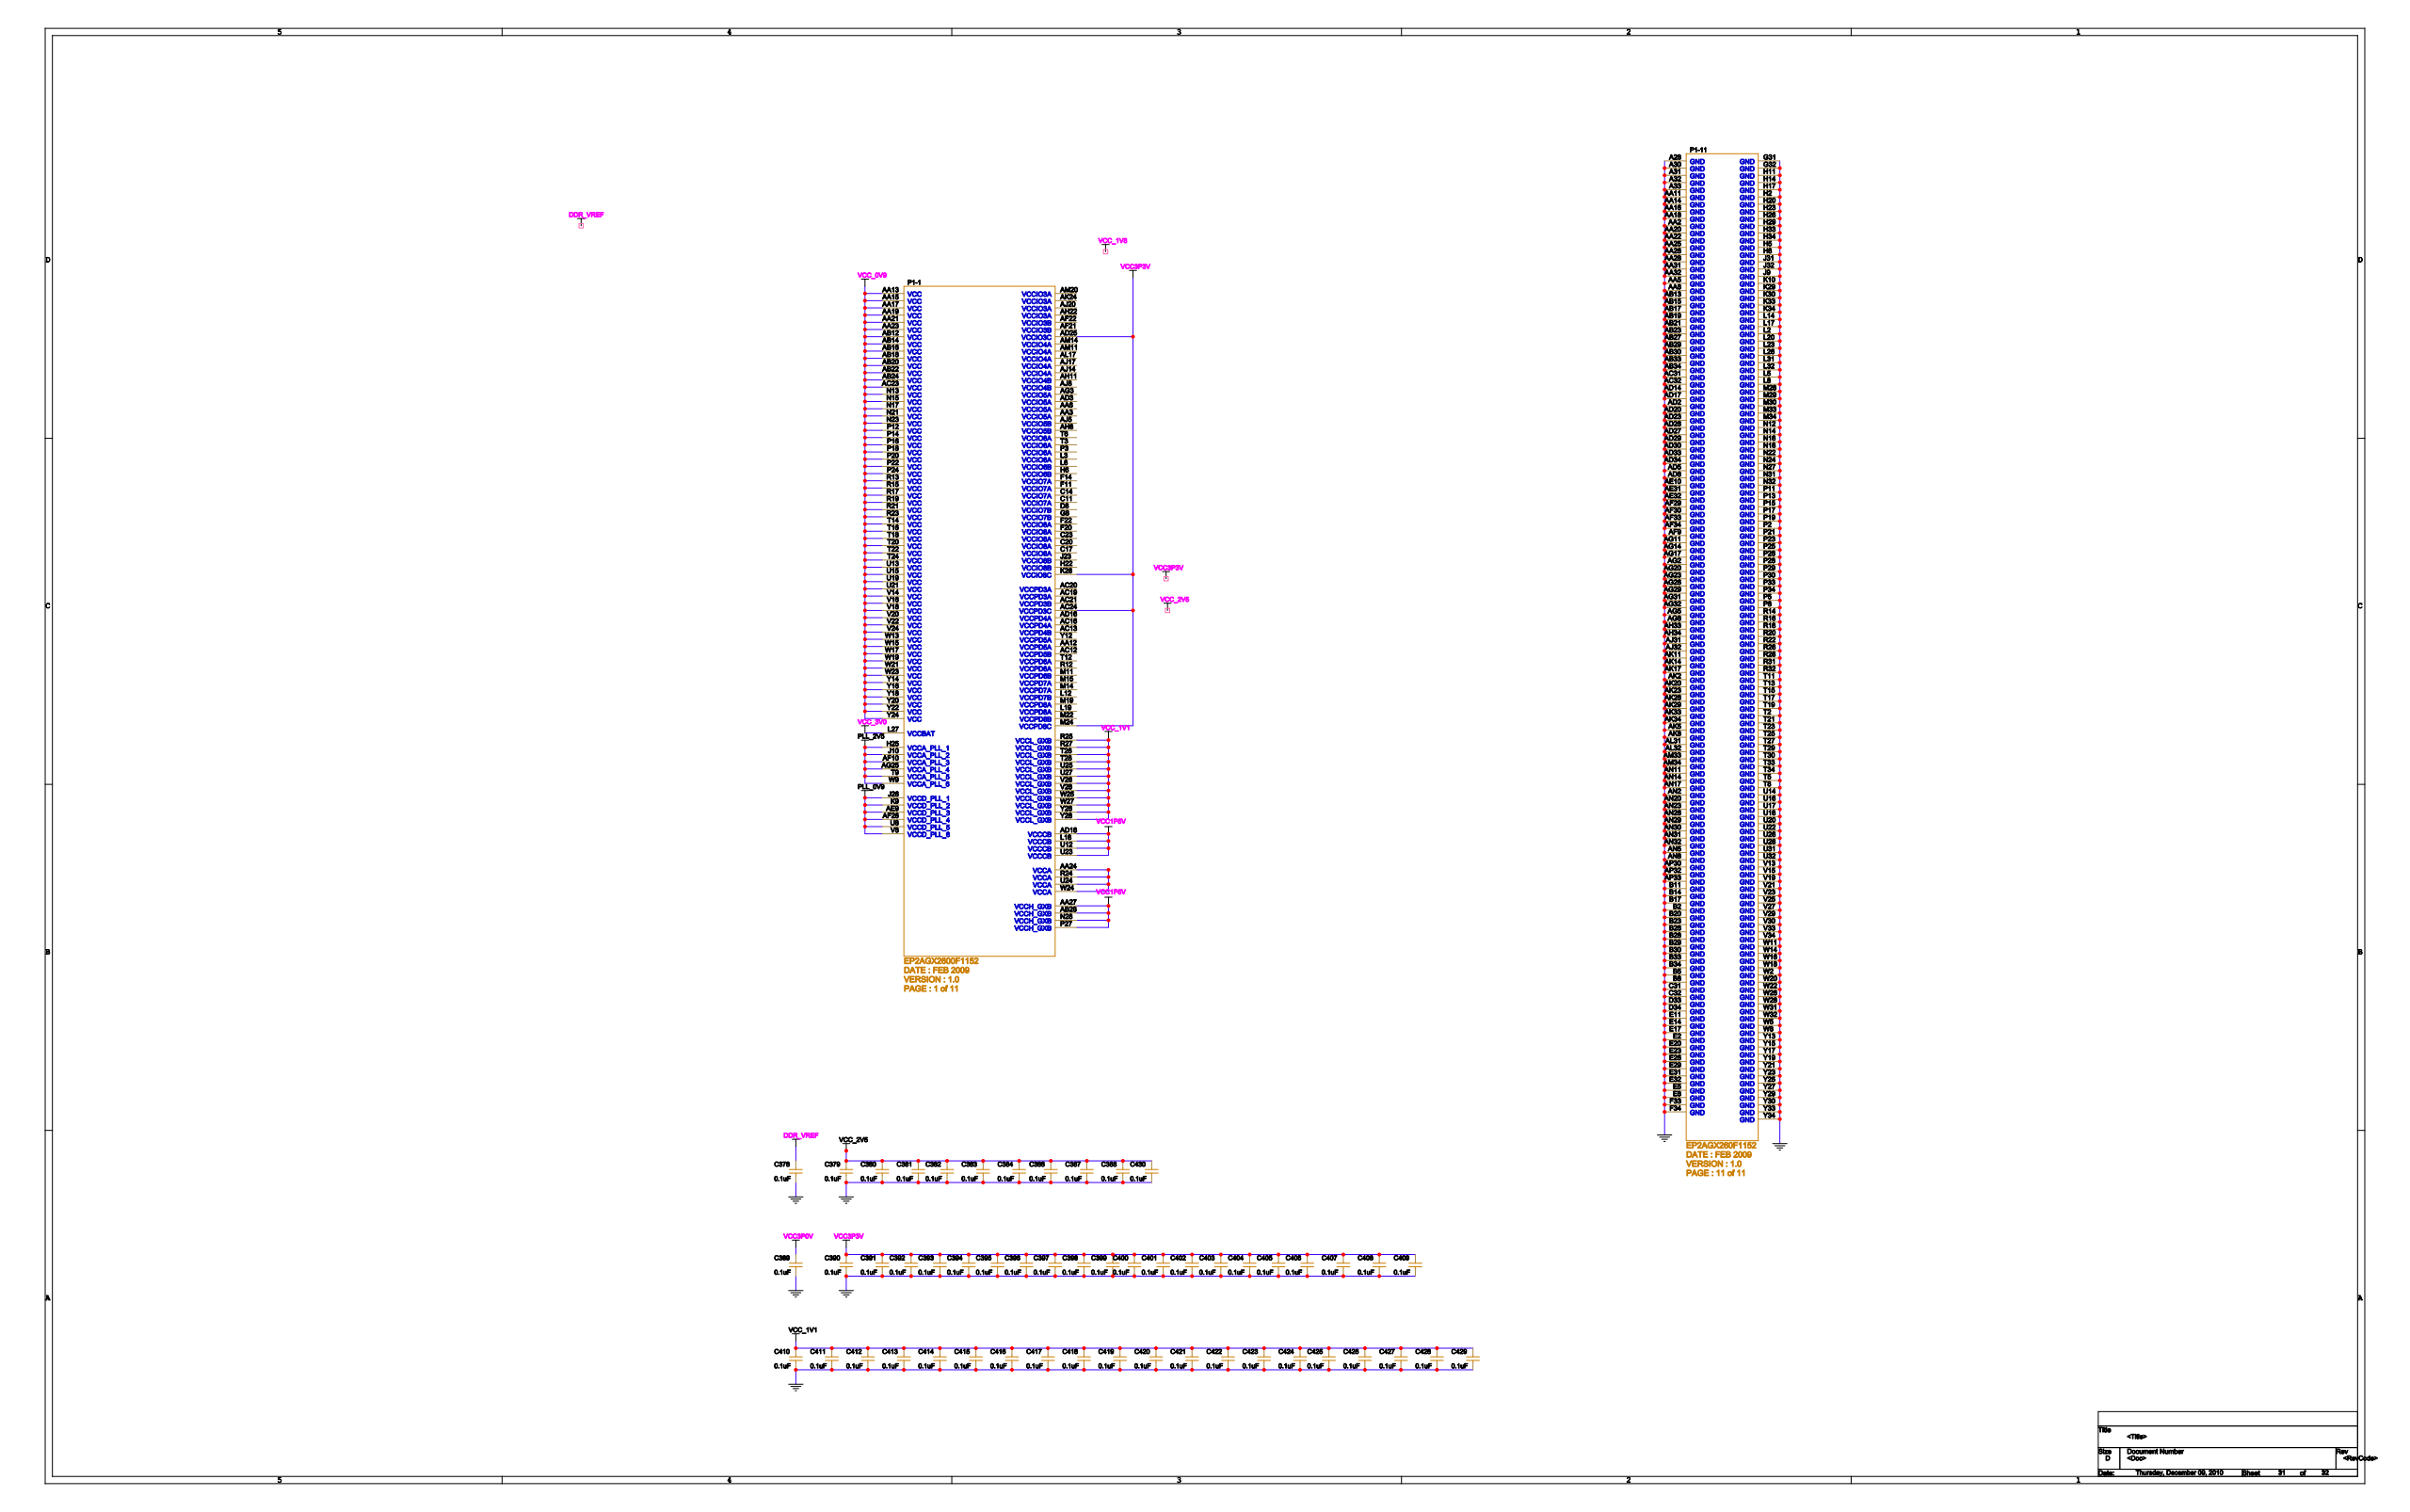Circuit board | Cadence Allegro | 1001 parts | 1318 nets | one sheet of the schematic
Parts on this sheet (reference | value | footprint):
C378 | 0.1uF | C0402
C379 | 0.1uF | C0402
C380 | 0.1uF | C0402
C381 | 0.1uF | C0402
C382 | 0.1uF | C0402
C383 | 0.1uF | C0402
C384 | 0.1uF | C0402
C386 | 0.1uF | C0402
C387 | 0.1uF | C0402
C388 | 0.1uF | C0402
C389 | 0.1uF | C0402
C390 | 0.1uF | C0402
C391 | 0.1uF | C0402
C392 | 0.1uF | C0402
C393 | 0.1uF | C0402
C394 | 0.1uF | C0402
C395 | 0.1uF | C0402
C396 | 0.1uF | C0402
C397 | 0.1uF | C0402
C398 | 0.1uF | C0402
C399 | 0.1uF | C0402
C400 | 0.1uF | C0402
C401 | 0.1uF | C0402
C402 | 0.1uF | C0402
C403 | 0.1uF | C0402
C404 | 0.1uF | C0402
C405 | 0.1uF | C0402
C406 | 0.1uF | C0402
C407 | 0.1uF | C0402
C408 | 0.1uF | C0402
C409 | 0.1uF | C0402
C410 | 0.1uF | C0402
C411 | 0.1uF | C0402
C412 | 0.1uF | C0402
C413 | 0.1uF | C0402
C414 | 0.1uF | C0402
C415 | 0.1uF | C0402
C416 | 0.1uF | C0402
C417 | 0.1uF | C0402
C418 | 0.1uF | C0402
C419 | 0.1uF | C0402
C420 | 0.1uF | C0402
C421 | 0.1uF | C0402
C422 | 0.1uF | C0402
C423 | 0.1uF | C0402
C424 | 0.1uF | C0402
C425 | 0.1uF | C0402
C426 | 0.1uF | C0402
C427 | 0.1uF | C0402
C428 | 0.1uF | C0402
C429 | 0.1uF | C0402
C430 | 0.1uF | C0402
U8 | DP83848C | DP83848C_48LQFP
U14 | MT48LC16M16 | TSOP54
U15 | MT48LC16M16 | TSOP54
U16 | SoC_HTC_01 | L529_XIN
U17 | MT48LC32M16 | TSOP54
U20 | MT48LC16M16 | TSOP54
U21 | MT48LC16M16 | TSOP54
U22 | SoC_HTC_01 | L529_XIN
U23 | MT48LC32M16 | TSOP54
U26 | MT48LC16M16 | TSOP54
U27 | MT48LC16M16 | TSOP54
U28 | SoC_HTC_01 | L529_XIN
U32 | MT48LC16M16 | TSOP54
Nets of these parts (net: part-pin ...):
GND: C378-2 C379-2 C380-2 C381-2 C382-2 C383-2 C384-2 C386-2 C387-2 C388-2 C389-2 C390-2 C391-2 C392-2 C393-2 C394-2 C395-2 C396-2 C397-2 C398-2 C399-2 C400-2 C401-2 C402-2 C403-2 C404-2 C405-2 C406-2 C407-2 C408-2 C409-2 C410-2 C411-2 C412-2 C413-2 C414-2 C415-2 C416-2 C417-2 C418-2 C419-2 C420-2 C421-2 C422-2 C423-2 C424-2 C425-2 C426-2 C427-2 C428-2 C429-2 C430-2 U16-AA3 U16-AA11 U16-AA12 U16-AA16 U16-AA18 U16-C11 U16-F22 U16-H22 U16-H23 U16-L5 U16-L6 U16-L18 U16-N18 U16-N21 U16-N23 U16-P3 U16-P16 U16-P18 U16-R16 U16-R18 U16-T5 U16-T9 U16-T17 U16-U8 U16-U17 U16-V18 U16-W13 U16-W15 U16-W16 U16-W18 U16-Y14 U16-Y15 U16-Y19 U22-AA3 U22-AA11 U22-AA12 U22-AA16 U22-AA18 U22-C11 U22-F22 U22-H22 U22-H23 U22-L5 U22-L6 U22-L18 U22-N18 U22-N21 U22-N23 U22-P3 U22-P16 U22-P18 U22-R16 U22-R18 U22-T5 U22-T9 U22-T17 U22-U8 U22-U17 U22-V18 U22-W13 U22-W15 U22-W16 U22-W18 U22-Y14 U22-Y15 U22-Y19 U28-AA3 U28-AA11 U28-AA12 U28-AA16 U28-AA18 U28-C11 U28-F22 U28-H22 U28-H23 U28-L5 U28-L6 U28-L18 U28-N18 U28-N21 U28-N23 U28-P3 U28-P16 U28-P18 U28-R16 U28-R18 U28-T5 U28-T9 U28-T17 U28-U8 U28-U17 U28-V18 U28-W13 U28-W15 U28-W16 U28-W18 U28-Y14 U28-Y15 U28-Y19
VCC_1V1: C410-1 C411-1 C412-1 C413-1 C414-1 C415-1 C416-1 C417-1 C418-1 C419-1 C420-1 C421-1 C422-1 C423-1 C424-1 C425-1 C426-1 C427-1 C428-1 C429-1
VCC3P0V: C389-1
VCC_2V5: C379-1 C380-1 C381-1 C382-1 C383-1 C384-1 C386-1 C387-1 C388-1 C430-1
VCC3P3V: C390-1 C391-1 C392-1 C393-1 C394-1 C395-1 C396-1 C397-1 C398-1 C399-1 C400-1 C401-1 C402-1 C403-1 C404-1 C405-1 C406-1 C407-1 C408-1 C409-1 U8-22 U8-32 U14-1 U15-1 U16-AA14 U16-B5 U16-E11 U16-H6 U16-H14 U16-L17 U16-P15 U16-R17 U16-T3 U16-T18 U16-W19 U16-Y12 U16-Y13 U16-Y16 U16-Y17 U17-1 U20-1 U21-1 U22-AA14 U22-B5 U22-E11 U22-H6 U22-H14 U22-L17 U22-P15 U22-R17 U22-T3 U22-T18 U22-W19 U22-Y12 U22-Y13 U22-Y16 U22-Y17 U23-1 U26-1 U27-1 U28-AA14 U28-B5 U28-E11 U28-H6 U28-H14 U28-L17 U28-P15 U28-R17 U28-T3 U28-T18 U28-W19 U28-Y12 U28-Y13 U28-Y16 U28-Y17 U32-1
DDR_VREF: C378-1